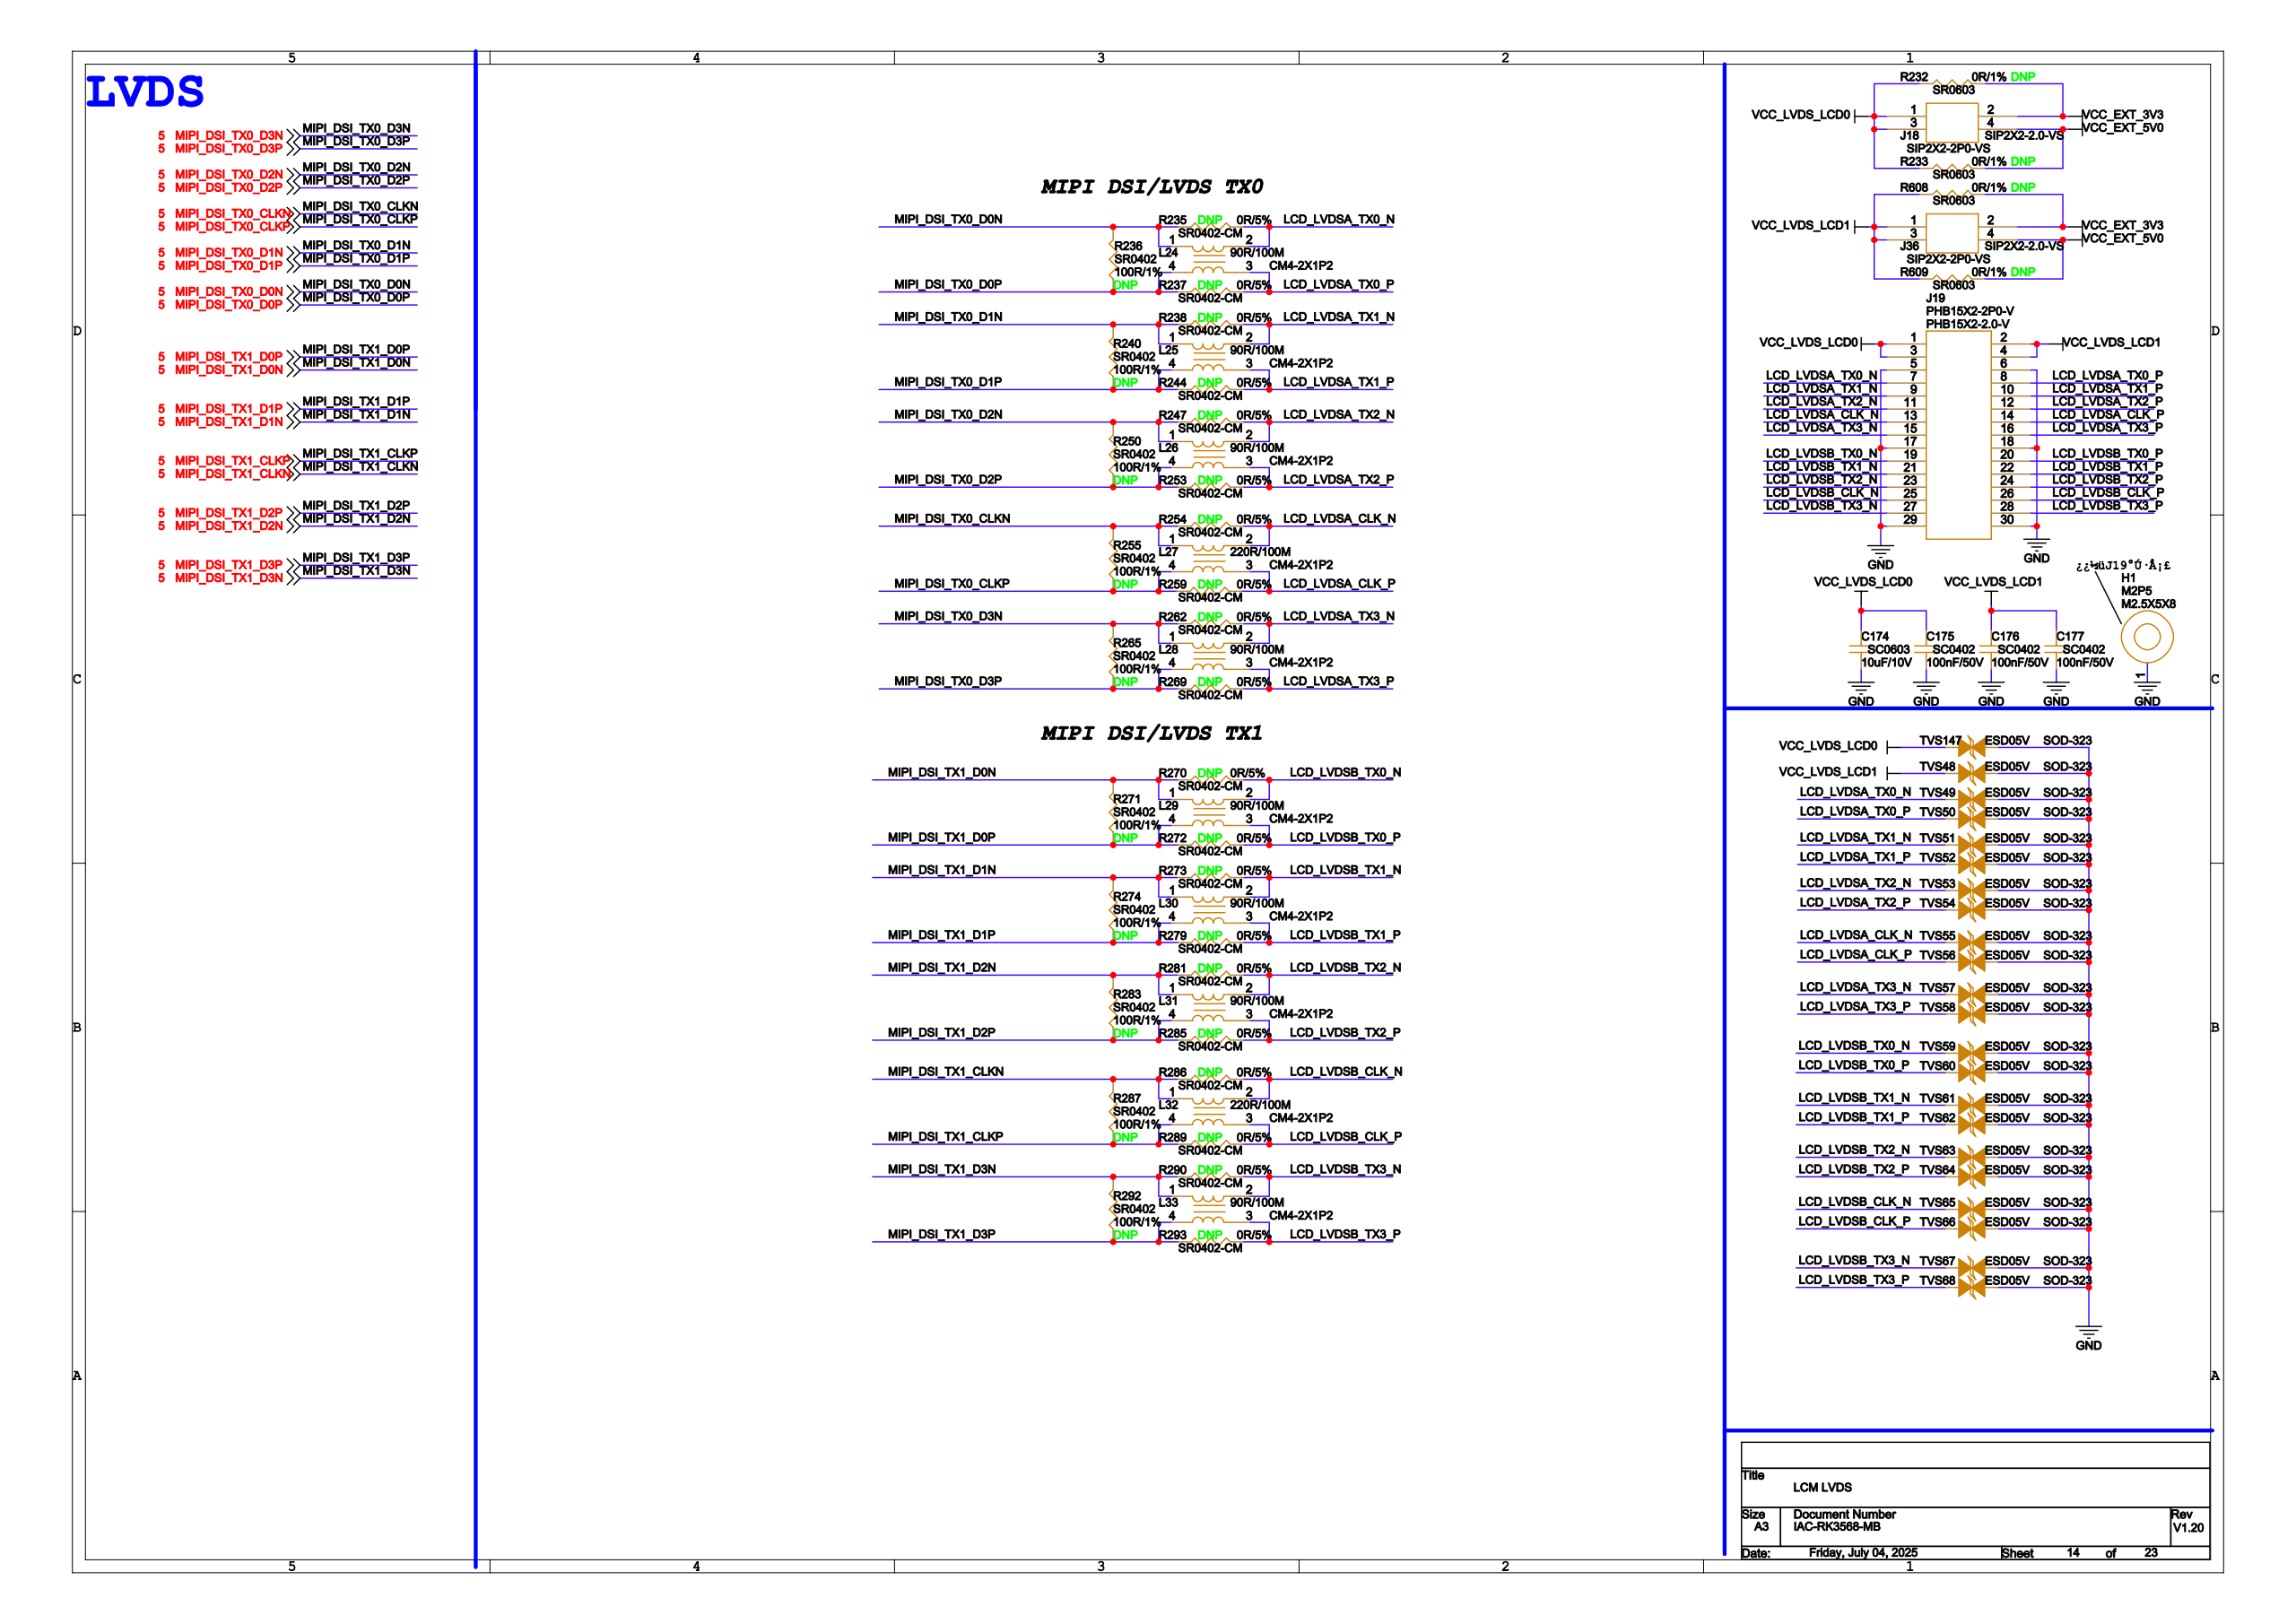Circuit board | Cadence Allegro | 1138 parts | 722 nets | one sheet of the schematic
Parts on this sheet (reference | value | footprint):
C174 | 10uF/10V | SC0603
C175 | 100nF/50V | SC0402
C176 | 100nF/50V | SC0402
C177 | 100nF/50V | SC0402
H1 | M2.5X5X8 | M2P5
J18 | SIP2X2-2.0-VS | SIP2X2-2P0-VS
J19 | PHB15X2-2.0-V | PHB15X2-2P0-V
J36 | SIP2X2-2.0-VS | SIP2X2-2P0-VS
L24 | 90R/100M | CM4-2X1P2
L25 | 90R/100M | CM4-2X1P2
L26 | 90R/100M | CM4-2X1P2
L27 | 220R/100M | CM4-2X1P2
L28 | 90R/100M | CM4-2X1P2
L29 | 90R/100M | CM4-2X1P2
L30 | 90R/100M | CM4-2X1P2
L31 | 90R/100M | CM4-2X1P2
L32 | 220R/100M | CM4-2X1P2
L33 | 90R/100M | CM4-2X1P2
R232 | 0R/1% | SR0603
R233 | 0R/1% | SR0603
R235 | 0R/5% | SR0402-CM
R236 | 100R/1% | SR0402
R237 | 0R/5% | SR0402-CM
R238 | 0R/5% | SR0402-CM
R240 | 100R/1% | SR0402
R244 | 0R/5% | SR0402-CM
R247 | 0R/5% | SR0402-CM
R250 | 100R/1% | SR0402
R253 | 0R/5% | SR0402-CM
R254 | 0R/5% | SR0402-CM
R255 | 100R/1% | SR0402
R259 | 0R/5% | SR0402-CM
R262 | 0R/5% | SR0402-CM
R265 | 100R/1% | SR0402
R269 | 0R/5% | SR0402-CM
R270 | 0R/5% | SR0402-CM
R271 | 100R/1% | SR0402
R272 | 0R/5% | SR0402-CM
R273 | 0R/5% | SR0402-CM
R274 | 100R/1% | SR0402
R279 | 0R/5% | SR0402-CM
R281 | 0R/5% | SR0402-CM
R283 | 100R/1% | SR0402
R285 | 0R/5% | SR0402-CM
R286 | 0R/5% | SR0402-CM
R287 | 100R/1% | SR0402
R289 | 0R/5% | SR0402-CM
R290 | 0R/5% | SR0402-CM
R292 | 100R/1% | SR0402
R293 | 0R/5% | SR0402-CM
R608 | 0R/1% | SR0603
R609 | 0R/1% | SR0603
TVS48 | ESD05V | SOD-323
TVS49 | ESD05V | SOD-323
TVS50 | ESD05V | SOD-323
TVS51 | ESD05V | SOD-323
TVS52 | ESD05V | SOD-323
TVS53 | ESD05V | SOD-323
TVS54 | ESD05V | SOD-323
TVS55 | ESD05V | SOD-323
TVS56 | ESD05V | SOD-323
TVS57 | ESD05V | SOD-323
TVS58 | ESD05V | SOD-323
TVS59 | ESD05V | SOD-323
TVS60 | ESD05V | SOD-323
TVS61 | ESD05V | SOD-323
TVS62 | ESD05V | SOD-323
TVS63 | ESD05V | SOD-323
TVS64 | ESD05V | SOD-323
TVS65 | ESD05V | SOD-323
TVS66 | ESD05V | SOD-323
TVS67 | ESD05V | SOD-323
TVS68 | ESD05V | SOD-323
TVS147 | ESD05V | SOD-323
Nets of these parts (net: part-pin ...):
VCC_EXT_5V0: J18-4 J36-4 R233-2 R609-2
VCC_EXT_3V3: J18-2 J36-2 R232-2 R608-2
GND: C174-2 C175-2 C176-2 C177-2 H1-1 TVS48-2 TVS49-2 TVS50-2 TVS51-2 TVS52-2 TVS53-2 TVS54-2 TVS55-2 TVS56-2 TVS57-2 TVS58-2 TVS59-2 TVS60-2 TVS61-2 TVS62-2 TVS63-2 TVS64-2 TVS65-2 TVS66-2 TVS67-2 TVS68-2 TVS147-2 J19-5 J19-6 J19-17 J19-18
VCC_LVDS_LCD0: C174-1 C175-1 J18-1 J18-3 R232-1 R233-1 TVS147-1 J19-1 J19-3
VCC_LVDS_LCD1: C176-1 C177-1 J36-1 J36-3 R608-1 R609-1 TVS48-1 J19-2 J19-4
LCD_LVDSA_TX0_N: L24-2 R235-2 TVS49-1 J19-7
LCD_LVDSA_TX0_P: L24-3 R237-2 TVS50-1 J19-8
LCD_LVDSA_TX1_N: L25-2 R238-2 TVS51-1 J19-9
LCD_LVDSA_TX1_P: L25-3 R244-2 TVS52-1 J19-10
LCD_LVDSA_TX2_N: L26-2 R247-2 TVS53-1 J19-11
LCD_LVDSA_TX2_P: L26-3 R253-2 TVS54-1 J19-12
LCD_LVDSA_CLK_N: L27-2 R254-2 TVS55-1 J19-13
LCD_LVDSA_CLK_P: L27-3 R259-2 TVS56-1 J19-14
LCD_LVDSA_TX3_N: L28-2 R262-2 TVS57-1 J19-15
LCD_LVDSA_TX3_P: L28-3 R269-2 TVS58-1 J19-16
LCD_LVDSB_TX0_N: L29-2 R270-2 TVS59-1 J19-19
LCD_LVDSB_TX0_P: L29-3 R272-2 TVS60-1 J19-20
LCD_LVDSB_TX1_N: L30-2 R273-2 TVS61-1 J19-21
LCD_LVDSB_TX1_P: L30-3 R279-2 TVS62-1 J19-22
LCD_LVDSB_TX2_N: L31-2 R281-2 TVS63-1 J19-23
LCD_LVDSB_TX2_P: L31-3 R285-2 TVS64-1 J19-24
LCD_LVDSB_CLK_N: L32-2 R286-2 TVS65-1 J19-25
LCD_LVDSB_CLK_P: L32-3 R289-2 TVS66-1 J19-26
LCD_LVDSB_TX3_N: L33-2 R290-2 TVS67-1 J19-27
LCD_LVDSB_TX3_P: L33-3 R293-2 TVS68-1 J19-28
MIPI_DSI_TX0_CLKN: L27-1 R254-1 R255-2
MIPI_DSI_TX0_CLKP: L27-4 R255-1 R259-1
MIPI_DSI_TX1_CLKN: L32-1 R286-1 R287-2
MIPI_DSI_TX1_CLKP: L32-4 R287-1 R289-1
MIPI_DSI_TX0_D0N: L24-1 R235-1 R236-2
MIPI_DSI_TX0_D0P: L24-4 R236-1 R237-1
MIPI_DSI_TX0_D1N: L25-1 R238-1 R240-2
MIPI_DSI_TX0_D1P: L25-4 R240-1 R244-1
MIPI_DSI_TX0_D2N: L26-1 R247-1 R250-2
MIPI_DSI_TX0_D2P: L26-4 R250-1 R253-1
MIPI_DSI_TX0_D3N: L28-1 R262-1 R265-2
MIPI_DSI_TX0_D3P: L28-4 R265-1 R269-1
MIPI_DSI_TX1_D0N: L29-1 R270-1 R271-2
MIPI_DSI_TX1_D0P: L29-4 R271-1 R272-1
MIPI_DSI_TX1_D1N: L30-1 R273-1 R274-2
MIPI_DSI_TX1_D1P: L30-4 R274-1 R279-1
MIPI_DSI_TX1_D2N: L31-1 R281-1 R283-2
MIPI_DSI_TX1_D2P: L31-4 R283-1 R285-1
MIPI_DSI_TX1_D3N: L33-1 R290-1 R292-2
MIPI_DSI_TX1_D3P: L33-4 R292-1 R293-1